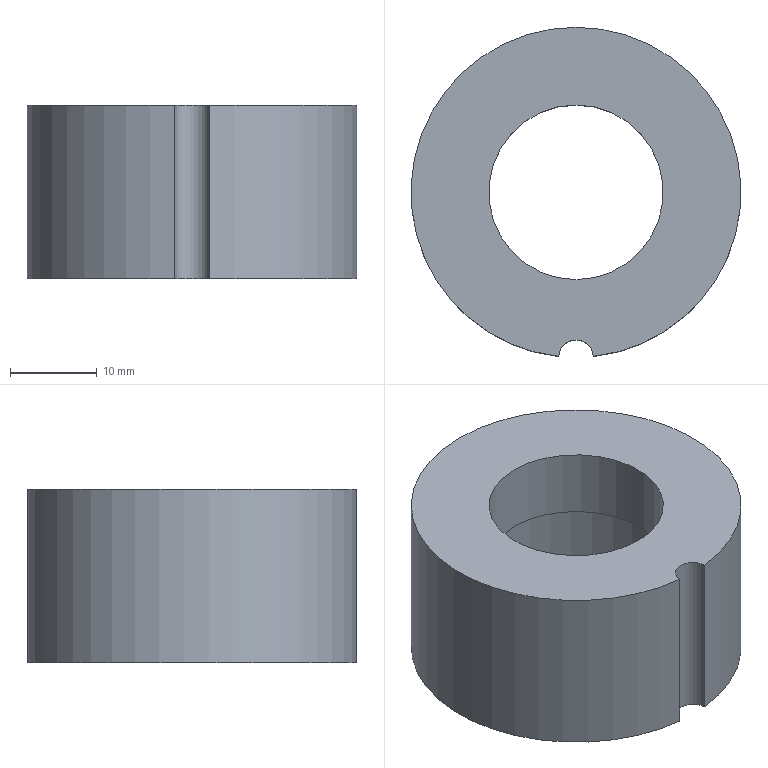Part | NX | features solid 2 | 1 solid | 7 faces | box 38 x 37.895 x 20 mm | volume 13352 mm3 | cylinder 4 | plane 3 | commonest cylinder face diameters 4 x1 20.1 x1 26.6 x1 38 x1
STEP:
#1=CARTESIAN_POINT('',(327.011,-224.352,-33.));
#2=VERTEX_POINT('',#1);
#3=CARTESIAN_POINT('',(327.011,-224.352,-13.));
#4=VERTEX_POINT('',#3);
#5=CARTESIAN_POINT('',(327.011,-224.352,-23.));
#6=DIRECTION('',(0.,0.,1.));
#7=VECTOR('',#6,1000.);
#8=LINE('',#5,#7);
#9=EDGE_CURVE('',#2,#4,#8,.T.);
#10=ORIENTED_EDGE('',*,*,#9,.F.);
#11=CARTESIAN_POINT('',(323.017,-224.352,-33.));
#12=VERTEX_POINT('',#11);
#13=CARTESIAN_POINT('',(325.014,-205.458,-33.));
#14=DIRECTION('',(0.,0.,1.));
#15=DIRECTION('',(0.,-1.,0.));
#16=AXIS2_PLACEMENT_3D('',#13,#14,#15);
#17=CIRCLE('',#16,19.);
#18=EDGE_CURVE('',#2,#12,#17,.T.);
#19=ORIENTED_EDGE('',*,*,#18,.T.);
#20=CARTESIAN_POINT('',(323.017,-224.352,-13.));
#21=VERTEX_POINT('',#20);
#22=CARTESIAN_POINT('',(323.017,-224.352,-23.));
#23=DIRECTION('',(0.,0.,1.));
#24=VECTOR('',#23,1000.);
#25=LINE('',#22,#24);
#26=EDGE_CURVE('',#21,#12,#25,.F.);
#27=ORIENTED_EDGE('',*,*,#26,.F.);
#28=CARTESIAN_POINT('',(325.014,-205.458,-13.));
#29=DIRECTION('',(0.,0.,1.));
#30=DIRECTION('',(0.,-1.,0.));
#31=AXIS2_PLACEMENT_3D('',#28,#29,#30);
#32=CIRCLE('',#31,19.);
#33=EDGE_CURVE('',#4,#21,#32,.T.);
#34=ORIENTED_EDGE('',*,*,#33,.F.);
#35=EDGE_LOOP('',(#10,#19,#27,#34));
#36=FACE_BOUND('',#35,.T.);
#37=CARTESIAN_POINT('',(325.014,-205.458,-33.));
#38=DIRECTION('',(0.,0.,1.));
#39=DIRECTION('',(0.,-1.,0.));
#40=AXIS2_PLACEMENT_3D('',#37,#38,#39);
#41=CYLINDRICAL_SURFACE('',#40,19.);
#42=ADVANCED_FACE('',(#36),#41,.T.);
#43=CARTESIAN_POINT('',(325.014,-218.758,-33.));
#44=VERTEX_POINT('',#43);
#45=CARTESIAN_POINT('',(325.014,-205.458,-33.));
#46=DIRECTION('',(0.,0.,1.));
#47=DIRECTION('',(0.,-1.,0.));
#48=AXIS2_PLACEMENT_3D('',#45,#46,#47);
#49=CIRCLE('',#48,13.3);
#50=EDGE_CURVE('',#44,#44,#49,.T.);
#51=ORIENTED_EDGE('',*,*,#50,.T.);
#52=EDGE_LOOP('',(#51));
#53=FACE_BOUND('',#52,.T.);
#54=ORIENTED_EDGE('',*,*,#18,.F.);
#55=CARTESIAN_POINT('',(325.014,-224.458,-33.));
#56=DIRECTION('',(0.,0.,1.));
#57=DIRECTION('',(0.,-1.,0.));
#58=AXIS2_PLACEMENT_3D('',#55,#56,#57);
#59=CIRCLE('',#58,2.);
#60=EDGE_CURVE('',#2,#12,#59,.T.);
#61=ORIENTED_EDGE('',*,*,#60,.T.);
#62=EDGE_LOOP('',(#54,#61));
#63=FACE_BOUND('',#62,.T.);
#64=CARTESIAN_POINT('',(325.014,-205.458,-33.));
#65=DIRECTION('',(0.,0.,1.));
#66=DIRECTION('',(0.,-1.,0.));
#67=AXIS2_PLACEMENT_3D('',#64,#65,#66);
#68=PLANE('',#67);
#69=ADVANCED_FACE('',(#53,#63),#68,.F.);
#70=CARTESIAN_POINT('',(325.014,-215.508,-13.));
#71=VERTEX_POINT('',#70);
#72=CARTESIAN_POINT('',(325.014,-205.458,-13.));
#73=DIRECTION('',(0.,0.,1.));
#74=DIRECTION('',(0.,-1.,0.));
#75=AXIS2_PLACEMENT_3D('',#72,#73,#74);
#76=CIRCLE('',#75,10.05);
#77=EDGE_CURVE('',#71,#71,#76,.T.);
#78=ORIENTED_EDGE('',*,*,#77,.F.);
#79=EDGE_LOOP('',(#78));
#80=FACE_BOUND('',#79,.T.);
#81=CARTESIAN_POINT('',(325.014,-224.458,-13.));
#82=DIRECTION('',(0.,0.,1.));
#83=DIRECTION('',(0.,-1.,0.));
#84=AXIS2_PLACEMENT_3D('',#81,#82,#83);
#85=CIRCLE('',#84,2.);
#86=EDGE_CURVE('',#4,#21,#85,.T.);
#87=ORIENTED_EDGE('',*,*,#86,.F.);
#88=ORIENTED_EDGE('',*,*,#33,.T.);
#89=EDGE_LOOP('',(#87,#88));
#90=FACE_BOUND('',#89,.T.);
#91=CARTESIAN_POINT('',(325.014,-205.458,-13.));
#92=DIRECTION('',(0.,0.,1.));
#93=DIRECTION('',(0.,-1.,0.));
#94=AXIS2_PLACEMENT_3D('',#91,#92,#93);
#95=PLANE('',#94);
#96=ADVANCED_FACE('',(#80,#90),#95,.T.);
#97=ORIENTED_EDGE('',*,*,#50,.F.);
#98=EDGE_LOOP('',(#97));
#99=FACE_BOUND('',#98,.T.);
#100=CARTESIAN_POINT('',(325.014,-218.758,-21.));
#101=VERTEX_POINT('',#100);
#102=CARTESIAN_POINT('',(325.014,-205.458,-21.));
#103=DIRECTION('',(0.,0.,1.));
#104=DIRECTION('',(0.,-1.,0.));
#105=AXIS2_PLACEMENT_3D('',#102,#103,#104);
#106=CIRCLE('',#105,13.3);
#107=EDGE_CURVE('',#101,#101,#106,.T.);
#108=ORIENTED_EDGE('',*,*,#107,.T.);
#109=EDGE_LOOP('',(#108));
#110=FACE_BOUND('',#109,.T.);
#111=CARTESIAN_POINT('',(325.014,-205.458,-33.));
#112=DIRECTION('',(0.,0.,1.));
#113=DIRECTION('',(0.,-1.,0.));
#114=AXIS2_PLACEMENT_3D('',#111,#112,#113);
#115=CYLINDRICAL_SURFACE('',#114,13.3);
#116=ADVANCED_FACE('',(#99,#110),#115,.F.);
#117=CARTESIAN_POINT('',(325.014,-215.508,-21.));
#118=VERTEX_POINT('',#117);
#119=CARTESIAN_POINT('',(325.014,-205.458,-21.));
#120=DIRECTION('',(0.,0.,1.));
#121=DIRECTION('',(0.,-1.,0.));
#122=AXIS2_PLACEMENT_3D('',#119,#120,#121);
#123=CIRCLE('',#122,10.05);
#124=EDGE_CURVE('',#118,#118,#123,.T.);
#125=ORIENTED_EDGE('',*,*,#124,.T.);
#126=EDGE_LOOP('',(#125));
#127=FACE_BOUND('',#126,.T.);
#128=ORIENTED_EDGE('',*,*,#107,.F.);
#129=EDGE_LOOP('',(#128));
#130=FACE_BOUND('',#129,.T.);
#131=CARTESIAN_POINT('',(325.014,-205.458,-21.));
#132=DIRECTION('',(0.,0.,1.));
#133=DIRECTION('',(0.,-1.,0.));
#134=AXIS2_PLACEMENT_3D('',#131,#132,#133);
#135=PLANE('',#134);
#136=ADVANCED_FACE('',(#127,#130),#135,.F.);
#137=ORIENTED_EDGE('',*,*,#9,.T.);
#138=ORIENTED_EDGE('',*,*,#86,.T.);
#139=ORIENTED_EDGE('',*,*,#26,.T.);
#140=ORIENTED_EDGE('',*,*,#60,.F.);
#141=EDGE_LOOP('',(#137,#138,#139,#140));
#142=FACE_BOUND('',#141,.T.);
#143=CARTESIAN_POINT('',(325.014,-224.458,-33.));
#144=DIRECTION('',(0.,0.,1.));
#145=DIRECTION('',(0.,-1.,0.));
#146=AXIS2_PLACEMENT_3D('',#143,#144,#145);
#147=CYLINDRICAL_SURFACE('',#146,2.);
#148=ADVANCED_FACE('',(#142),#147,.F.);
#149=ORIENTED_EDGE('',*,*,#77,.T.);
#150=EDGE_LOOP('',(#149));
#151=FACE_BOUND('',#150,.T.);
#152=ORIENTED_EDGE('',*,*,#124,.F.);
#153=EDGE_LOOP('',(#152));
#154=FACE_BOUND('',#153,.T.);
#155=CARTESIAN_POINT('',(325.014,-205.458,-33.));
#156=DIRECTION('',(0.,0.,1.));
#157=DIRECTION('',(0.,-1.,0.));
#158=AXIS2_PLACEMENT_3D('',#155,#156,#157);
#159=CYLINDRICAL_SURFACE('',#158,10.05);
#160=ADVANCED_FACE('',(#151,#154),#159,.F.);
#161=CLOSED_SHELL('',(#42,#69,#96,#116,#136,#148,#160));
#162=MANIFOLD_SOLID_BREP('',#161);
#163=(LENGTH_UNIT()NAMED_UNIT(*)SI_UNIT(.MILLI.,.METRE.));
#164=UNCERTAINTY_MEASURE_WITH_UNIT(LENGTH_MEASURE(0.00001),#163,'','');
#165=(NAMED_UNIT(*)PLANE_ANGLE_UNIT()SI_UNIT($,.RADIAN.));
#166=(NAMED_UNIT(*)SI_UNIT($,.STERADIAN.)SOLID_ANGLE_UNIT());
#167=(GEOMETRIC_REPRESENTATION_CONTEXT(3)GLOBAL_UNCERTAINTY_ASSIGNED_CONTEXT((#164))GLOBAL_UNIT_ASSIGNED_CONTEXT((#163,#165,#166))REPRESENTATION_CONTEXT('',''));
#168=ADVANCED_BREP_SHAPE_REPRESENTATION('',(#162),#167);